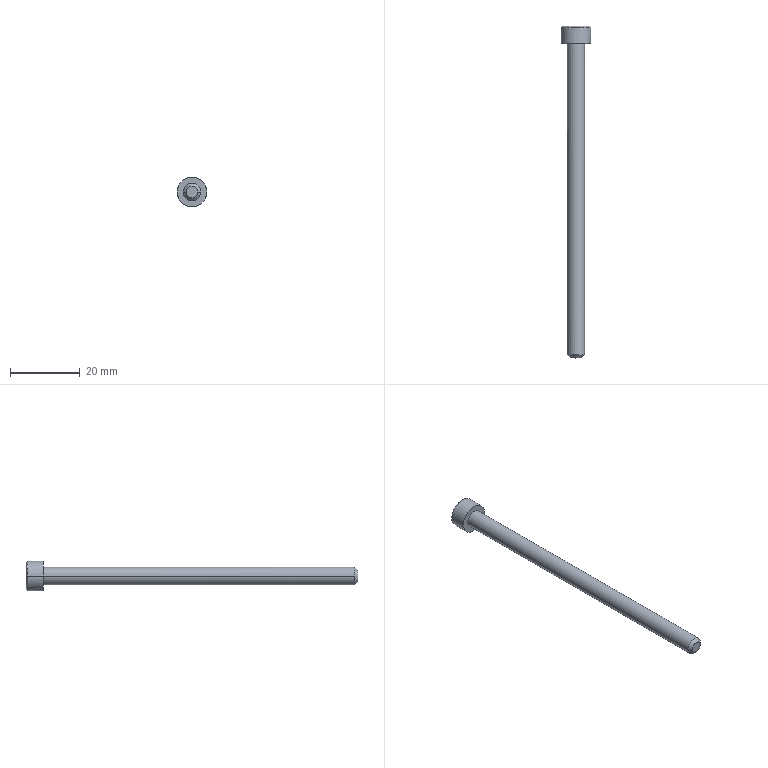Part | STEP file | BB62-M5-90L-6 | 1 solid | 18 faces | box 8.5 x 95 x 8.5 mm | volume 2008 mm3 | plane 10 | cylinder 4 | cone 4 | commonest cylinder face diameters 5 x2 8.5 x2
STEP:
#1=CARTESIAN_POINT('',(-4.25,0.,0.));
#2=VERTEX_POINT('',#1);
#3=CARTESIAN_POINT('',(4.25,0.,0.));
#4=VERTEX_POINT('',#3);
#5=CARTESIAN_POINT('',(0.,0.,0.));
#6=DIRECTION('',(0.,1.,0.));
#7=DIRECTION('',(-1.,0.,0.));
#8=AXIS2_PLACEMENT_3D('',#5,#6,#7);
#9=CIRCLE('',#8,4.25);
#10=EDGE_CURVE('',#2,#4,#9,.T.);
#11=ORIENTED_EDGE('',*,*,#10,.F.);
#12=CARTESIAN_POINT('',(0.,0.,0.));
#13=DIRECTION('',(0.,1.,0.));
#14=DIRECTION('',(1.,0.,0.));
#15=AXIS2_PLACEMENT_3D('',#12,#13,#14);
#16=CIRCLE('',#15,4.25);
#17=EDGE_CURVE('',#4,#2,#16,.T.);
#18=ORIENTED_EDGE('',*,*,#17,.F.);
#19=EDGE_LOOP('',(#11,#18));
#20=FACE_OUTER_BOUND('',#19,.T.);
#21=CARTESIAN_POINT('',(-2.5,0.,0.));
#22=VERTEX_POINT('',#21);
#23=CARTESIAN_POINT('',(2.5,0.,0.));
#24=VERTEX_POINT('',#23);
#25=CARTESIAN_POINT('',(0.,0.,0.));
#26=DIRECTION('',(0.,1.,0.));
#27=DIRECTION('',(-1.,0.,0.));
#28=AXIS2_PLACEMENT_3D('',#25,#26,#27);
#29=CIRCLE('',#28,2.5);
#30=EDGE_CURVE('',#22,#24,#29,.T.);
#31=ORIENTED_EDGE('',*,*,#30,.T.);
#32=CARTESIAN_POINT('',(0.,0.,0.));
#33=DIRECTION('',(0.,1.,0.));
#34=DIRECTION('',(1.,0.,0.));
#35=AXIS2_PLACEMENT_3D('',#32,#33,#34);
#36=CIRCLE('',#35,2.5);
#37=EDGE_CURVE('',#24,#22,#36,.T.);
#38=ORIENTED_EDGE('',*,*,#37,.T.);
#39=EDGE_LOOP('',(#31,#38));
#40=FACE_BOUND('',#39,.T.);
#41=CARTESIAN_POINT('',(-9.016,0.,9.016));
#42=DIRECTION('',(0.,1.,0.));
#43=DIRECTION('',(1.,0.,0.));
#44=AXIS2_PLACEMENT_3D('',#41,#42,#43);
#45=PLANE('',#44);
#46=ADVANCED_FACE('',(#20,#40),#45,.F.);
#47=CARTESIAN_POINT('',(4.25,4.7,0.));
#48=VERTEX_POINT('',#47);
#49=CARTESIAN_POINT('',(4.25,0.,0.));
#50=DIRECTION('',(0.,1.,0.));
#51=VECTOR('',#50,1000.);
#52=LINE('',#49,#51);
#53=EDGE_CURVE('',#4,#48,#52,.T.);
#54=ORIENTED_EDGE('',*,*,#53,.F.);
#55=ORIENTED_EDGE('',*,*,#17,.T.);
#56=CARTESIAN_POINT('',(-4.25,4.7,0.));
#57=VERTEX_POINT('',#56);
#58=CARTESIAN_POINT('',(-4.25,0.,0.));
#59=DIRECTION('',(0.,1.,0.));
#60=VECTOR('',#59,1000.);
#61=LINE('',#58,#60);
#62=EDGE_CURVE('',#2,#57,#61,.T.);
#63=ORIENTED_EDGE('',*,*,#62,.T.);
#64=CARTESIAN_POINT('',(4.25,4.7,0.));
#65=CARTESIAN_POINT('',(4.25,4.7,-0.5563));
#66=CARTESIAN_POINT('',(4.139,4.7,-1.112));
#67=CARTESIAN_POINT('',(3.714,4.7,-2.14));
#68=CARTESIAN_POINT('',(3.399,4.7,-2.612));
#69=CARTESIAN_POINT('',(2.612,4.7,-3.399));
#70=CARTESIAN_POINT('',(2.14,4.7,-3.714));
#71=CARTESIAN_POINT('',(1.112,4.7,-4.139));
#72=CARTESIAN_POINT('',(0.5563,4.7,-4.25));
#73=CARTESIAN_POINT('',(-0.5563,4.7,-4.25));
#74=CARTESIAN_POINT('',(-1.112,4.7,-4.139));
#75=CARTESIAN_POINT('',(-2.14,4.7,-3.714));
#76=CARTESIAN_POINT('',(-2.612,4.7,-3.399));
#77=CARTESIAN_POINT('',(-3.399,4.7,-2.612));
#78=CARTESIAN_POINT('',(-3.714,4.7,-2.14));
#79=CARTESIAN_POINT('',(-4.139,4.7,-1.112));
#80=CARTESIAN_POINT('',(-4.25,4.7,-0.5563));
#81=CARTESIAN_POINT('',(-4.25,4.7,0.));
#82=B_SPLINE_CURVE_WITH_KNOTS('',3,(#64,#65,#66,#67,#68,#69,#70,#71,#72,#73,#74,#75,#76,#77,#78,#79,#80,#81),.UNSPECIFIED.,.F.,.F.,(4,2,2,2,2,2,2,2,4),(0.,0.125,0.25,0.375,0.5,0.625,0.75,0.875,1.),.UNSPECIFIED.);
#83=EDGE_CURVE('',#48,#57,#82,.T.);
#84=ORIENTED_EDGE('',*,*,#83,.F.);
#85=EDGE_LOOP('',(#54,#55,#63,#84));
#86=FACE_OUTER_BOUND('',#85,.T.);
#87=CARTESIAN_POINT('',(0.,2.35,0.));
#88=DIRECTION('',(0.,1.,0.));
#89=DIRECTION('',(1.,0.,0.));
#90=AXIS2_PLACEMENT_3D('',#87,#88,#89);
#91=CYLINDRICAL_SURFACE('',#90,4.25);
#92=ADVANCED_FACE('',(#86),#91,.T.);
#93=CARTESIAN_POINT('',(3.73,5.,0.));
#94=VERTEX_POINT('',#93);
#95=CARTESIAN_POINT('',(3.73,5.,0.));
#96=CARTESIAN_POINT('',(3.904,4.9,0.));
#97=CARTESIAN_POINT('',(4.077,4.8,0.));
#98=CARTESIAN_POINT('',(4.25,4.7,0.));
#99=B_SPLINE_CURVE_WITH_KNOTS('',3,(#95,#96,#97,#98),.UNSPECIFIED.,.F.,.F.,(4,4),(0.,1.),.UNSPECIFIED.);
#100=EDGE_CURVE('',#94,#48,#99,.T.);
#101=ORIENTED_EDGE('',*,*,#100,.T.);
#102=ORIENTED_EDGE('',*,*,#83,.T.);
#103=CARTESIAN_POINT('',(-3.73,5.,0.));
#104=VERTEX_POINT('',#103);
#105=CARTESIAN_POINT('',(-3.73,5.,0.));
#106=CARTESIAN_POINT('',(-3.904,4.9,0.));
#107=CARTESIAN_POINT('',(-4.077,4.8,0.));
#108=CARTESIAN_POINT('',(-4.25,4.7,0.));
#109=B_SPLINE_CURVE_WITH_KNOTS('',3,(#105,#106,#107,#108),.UNSPECIFIED.,.F.,.F.,(4,4),(0.,1.),.UNSPECIFIED.);
#110=EDGE_CURVE('',#104,#57,#109,.T.);
#111=ORIENTED_EDGE('',*,*,#110,.F.);
#112=CARTESIAN_POINT('',(3.73,5.,0.));
#113=CARTESIAN_POINT('',(3.742,5.,-0.9708));
#114=CARTESIAN_POINT('',(3.325,5.,-1.947));
#115=CARTESIAN_POINT('',(2.293,5.,-2.984));
#116=CARTESIAN_POINT('',(1.881,5.,-3.259));
#117=CARTESIAN_POINT('',(0.9786,5.,-3.631));
#118=CARTESIAN_POINT('',(0.,5.,-3.829));
#119=CARTESIAN_POINT('',(-0.9786,5.,-3.631));
#120=CARTESIAN_POINT('',(-1.881,5.,-3.259));
#121=CARTESIAN_POINT('',(-2.293,5.,-2.984));
#122=CARTESIAN_POINT('',(-3.325,5.,-1.947));
#123=CARTESIAN_POINT('',(-3.742,5.,-0.9708));
#124=CARTESIAN_POINT('',(-3.73,5.,0.));
#125=B_SPLINE_CURVE_WITH_KNOTS('',3,(#112,#113,#114,#115,#116,#117,#118,#119,#120,#121,#122,#123,#124),.UNSPECIFIED.,.F.,.F.,(4,2,2,1,2,2,4),(0.,0.25,0.375,0.5,0.625,0.75,1.),.UNSPECIFIED.);
#126=EDGE_CURVE('',#94,#104,#125,.T.);
#127=ORIENTED_EDGE('',*,*,#126,.F.);
#128=EDGE_LOOP('',(#101,#102,#111,#127));
#129=FACE_OUTER_BOUND('',#128,.T.);
#130=CARTESIAN_POINT('',(0.,-992.846,0.));
#131=DIRECTION('',(0.,-1.,0.));
#132=DIRECTION('',(0.,0.,1.));
#133=AXIS2_PLACEMENT_3D('',#130,#131,#132);
#134=CONICAL_SURFACE('',#133,1731.952,1.047);
#135=ADVANCED_FACE('',(#129),#134,.T.);
#136=CARTESIAN_POINT('',(-3.73,5.,0.));
#137=CARTESIAN_POINT('',(-3.742,5.,0.9708));
#138=CARTESIAN_POINT('',(-3.325,5.,1.947));
#139=CARTESIAN_POINT('',(-2.293,5.,2.984));
#140=CARTESIAN_POINT('',(-1.881,5.,3.259));
#141=CARTESIAN_POINT('',(-0.9786,5.,3.631));
#142=CARTESIAN_POINT('',(0.,5.,3.829));
#143=CARTESIAN_POINT('',(0.9786,5.,3.631));
#144=CARTESIAN_POINT('',(1.881,5.,3.259));
#145=CARTESIAN_POINT('',(2.293,5.,2.984));
#146=CARTESIAN_POINT('',(3.325,5.,1.947));
#147=CARTESIAN_POINT('',(3.742,5.,0.9708));
#148=CARTESIAN_POINT('',(3.73,5.,0.));
#149=B_SPLINE_CURVE_WITH_KNOTS('',3,(#136,#137,#138,#139,#140,#141,#142,#143,#144,#145,#146,#147,#148),.UNSPECIFIED.,.F.,.F.,(4,2,2,1,2,2,4),(0.,0.25,0.375,0.5,0.625,0.75,1.),.UNSPECIFIED.);
#150=EDGE_CURVE('',#104,#94,#149,.T.);
#151=ORIENTED_EDGE('',*,*,#150,.T.);
#152=ORIENTED_EDGE('',*,*,#126,.T.);
#153=EDGE_LOOP('',(#151,#152));
#154=FACE_OUTER_BOUND('',#153,.T.);
#155=CARTESIAN_POINT('',(2.,5.,1.155));
#156=VERTEX_POINT('',#155);
#157=CARTESIAN_POINT('',(2.,5.,-1.155));
#158=VERTEX_POINT('',#157);
#159=CARTESIAN_POINT('',(2.,5.,1.155));
#160=DIRECTION('',(0.,0.,-1.));
#161=VECTOR('',#160,1000.);
#162=LINE('',#159,#161);
#163=EDGE_CURVE('',#156,#158,#162,.T.);
#164=ORIENTED_EDGE('',*,*,#163,.F.);
#165=CARTESIAN_POINT('',(0.,5.,2.309));
#166=VERTEX_POINT('',#165);
#167=CARTESIAN_POINT('',(0.,5.,2.309));
#168=DIRECTION('',(0.866,0.,-0.5));
#169=VECTOR('',#168,1000.);
#170=LINE('',#167,#169);
#171=EDGE_CURVE('',#166,#156,#170,.T.);
#172=ORIENTED_EDGE('',*,*,#171,.F.);
#173=CARTESIAN_POINT('',(-2.,5.,1.155));
#174=VERTEX_POINT('',#173);
#175=CARTESIAN_POINT('',(-2.,5.,1.155));
#176=DIRECTION('',(0.866,0.,0.5));
#177=VECTOR('',#176,1000.);
#178=LINE('',#175,#177);
#179=EDGE_CURVE('',#174,#166,#178,.T.);
#180=ORIENTED_EDGE('',*,*,#179,.F.);
#181=CARTESIAN_POINT('',(-2.,5.,-1.155));
#182=VERTEX_POINT('',#181);
#183=CARTESIAN_POINT('',(-2.,5.,-1.155));
#184=DIRECTION('',(0.,0.,1.));
#185=VECTOR('',#184,1000.);
#186=LINE('',#183,#185);
#187=EDGE_CURVE('',#182,#174,#186,.T.);
#188=ORIENTED_EDGE('',*,*,#187,.F.);
#189=CARTESIAN_POINT('',(0.,5.,-2.309));
#190=VERTEX_POINT('',#189);
#191=CARTESIAN_POINT('',(0.,5.,-2.309));
#192=DIRECTION('',(-0.866,0.,0.5));
#193=VECTOR('',#192,1000.);
#194=LINE('',#191,#193);
#195=EDGE_CURVE('',#190,#182,#194,.T.);
#196=ORIENTED_EDGE('',*,*,#195,.F.);
#197=CARTESIAN_POINT('',(2.,5.,-1.155));
#198=DIRECTION('',(-0.866,0.,-0.5));
#199=VECTOR('',#198,1000.);
#200=LINE('',#197,#199);
#201=EDGE_CURVE('',#158,#190,#200,.T.);
#202=ORIENTED_EDGE('',*,*,#201,.F.);
#203=EDGE_LOOP('',(#164,#172,#180,#188,#196,#202));
#204=FACE_BOUND('',#203,.T.);
#205=CARTESIAN_POINT('',(-7.913,5.,7.913));
#206=DIRECTION('',(0.,1.,0.));
#207=DIRECTION('',(1.,0.,0.));
#208=AXIS2_PLACEMENT_3D('',#205,#206,#207);
#209=PLANE('',#208);
#210=ADVANCED_FACE('',(#154,#204),#209,.T.);
#211=ORIENTED_EDGE('',*,*,#110,.T.);
#212=CARTESIAN_POINT('',(-4.25,4.7,0.));
#213=CARTESIAN_POINT('',(-4.25,4.7,0.5563));
#214=CARTESIAN_POINT('',(-4.139,4.7,1.112));
#215=CARTESIAN_POINT('',(-3.714,4.7,2.14));
#216=CARTESIAN_POINT('',(-3.399,4.7,2.612));
#217=CARTESIAN_POINT('',(-2.612,4.7,3.399));
#218=CARTESIAN_POINT('',(-2.14,4.7,3.714));
#219=CARTESIAN_POINT('',(-1.112,4.7,4.139));
#220=CARTESIAN_POINT('',(-0.5563,4.7,4.25));
#221=CARTESIAN_POINT('',(0.5563,4.7,4.25));
#222=CARTESIAN_POINT('',(1.112,4.7,4.139));
#223=CARTESIAN_POINT('',(2.14,4.7,3.714));
#224=CARTESIAN_POINT('',(2.612,4.7,3.399));
#225=CARTESIAN_POINT('',(3.399,4.7,2.612));
#226=CARTESIAN_POINT('',(3.714,4.7,2.14));
#227=CARTESIAN_POINT('',(4.139,4.7,1.112));
#228=CARTESIAN_POINT('',(4.25,4.7,0.5563));
#229=CARTESIAN_POINT('',(4.25,4.7,0.));
#230=B_SPLINE_CURVE_WITH_KNOTS('',3,(#212,#213,#214,#215,#216,#217,#218,#219,#220,#221,#222,#223,#224,#225,#226,#227,#228,#229),.UNSPECIFIED.,.F.,.F.,(4,2,2,2,2,2,2,2,4),(0.,0.125,0.25,0.375,0.5,0.625,0.75,0.875,1.),.UNSPECIFIED.);
#231=EDGE_CURVE('',#57,#48,#230,.T.);
#232=ORIENTED_EDGE('',*,*,#231,.T.);
#233=ORIENTED_EDGE('',*,*,#100,.F.);
#234=ORIENTED_EDGE('',*,*,#150,.F.);
#235=EDGE_LOOP('',(#211,#232,#233,#234));
#236=FACE_OUTER_BOUND('',#235,.T.);
#237=CARTESIAN_POINT('',(0.,-992.846,0.));
#238=DIRECTION('',(0.,-1.,0.));
#239=DIRECTION('',(0.,0.,-1.));
#240=AXIS2_PLACEMENT_3D('',#237,#238,#239);
#241=CONICAL_SURFACE('',#240,1731.952,1.047);
#242=ADVANCED_FACE('',(#236),#241,.T.);
#243=ORIENTED_EDGE('',*,*,#62,.F.);
#244=ORIENTED_EDGE('',*,*,#10,.T.);
#245=ORIENTED_EDGE('',*,*,#53,.T.);
#246=ORIENTED_EDGE('',*,*,#231,.F.);
#247=EDGE_LOOP('',(#243,#244,#245,#246));
#248=FACE_OUTER_BOUND('',#247,.T.);
#249=CARTESIAN_POINT('',(0.,2.35,0.));
#250=DIRECTION('',(0.,1.,0.));
#251=DIRECTION('',(1.,0.,0.));
#252=AXIS2_PLACEMENT_3D('',#249,#250,#251);
#253=CYLINDRICAL_SURFACE('',#252,4.25);
#254=ADVANCED_FACE('',(#248),#253,.T.);
#255=CARTESIAN_POINT('',(0.,2.5,-2.309));
#256=VERTEX_POINT('',#255);
#257=CARTESIAN_POINT('',(0.,5.,-2.309));
#258=DIRECTION('',(0.,-1.,0.));
#259=VECTOR('',#258,1000.);
#260=LINE('',#257,#259);
#261=EDGE_CURVE('',#190,#256,#260,.T.);
#262=ORIENTED_EDGE('',*,*,#261,.T.);
#263=CARTESIAN_POINT('',(2.,2.5,-1.155));
#264=VERTEX_POINT('',#263);
#265=CARTESIAN_POINT('',(2.,2.5,-1.155));
#266=DIRECTION('',(-0.866,0.,-0.5));
#267=VECTOR('',#266,1000.);
#268=LINE('',#265,#267);
#269=EDGE_CURVE('',#264,#256,#268,.T.);
#270=ORIENTED_EDGE('',*,*,#269,.F.);
#271=CARTESIAN_POINT('',(2.,5.,-1.155));
#272=DIRECTION('',(0.,-1.,0.));
#273=VECTOR('',#272,1000.);
#274=LINE('',#271,#273);
#275=EDGE_CURVE('',#158,#264,#274,.T.);
#276=ORIENTED_EDGE('',*,*,#275,.F.);
#277=ORIENTED_EDGE('',*,*,#201,.T.);
#278=EDGE_LOOP('',(#262,#270,#276,#277));
#279=FACE_OUTER_BOUND('',#278,.T.);
#280=CARTESIAN_POINT('',(3.211,1.197,-0.4558));
#281=DIRECTION('',(0.5,0.,-0.866));
#282=DIRECTION('',(-0.866,0.,-0.5));
#283=AXIS2_PLACEMENT_3D('',#280,#281,#282);
#284=PLANE('',#283);
#285=ADVANCED_FACE('',(#279),#284,.F.);
#286=ORIENTED_EDGE('',*,*,#275,.T.);
#287=CARTESIAN_POINT('',(2.,2.5,1.155));
#288=VERTEX_POINT('',#287);
#289=CARTESIAN_POINT('',(2.,2.5,1.155));
#290=DIRECTION('',(0.,0.,-1.));
#291=VECTOR('',#290,1000.);
#292=LINE('',#289,#291);
#293=EDGE_CURVE('',#288,#264,#292,.T.);
#294=ORIENTED_EDGE('',*,*,#293,.F.);
#295=CARTESIAN_POINT('',(2.,5.,1.155));
#296=DIRECTION('',(0.,-1.,0.));
#297=VECTOR('',#296,1000.);
#298=LINE('',#295,#297);
#299=EDGE_CURVE('',#156,#288,#298,.T.);
#300=ORIENTED_EDGE('',*,*,#299,.F.);
#301=ORIENTED_EDGE('',*,*,#163,.T.);
#302=EDGE_LOOP('',(#286,#294,#300,#301));
#303=FACE_OUTER_BOUND('',#302,.T.);
#304=CARTESIAN_POINT('',(2.,1.197,2.553));
#305=DIRECTION('',(1.,0.,0.));
#306=DIRECTION('',(0.,0.,-1.));
#307=AXIS2_PLACEMENT_3D('',#304,#305,#306);
#308=PLANE('',#307);
#309=ADVANCED_FACE('',(#303),#308,.F.);
#310=ORIENTED_EDGE('',*,*,#299,.T.);
#311=CARTESIAN_POINT('',(0.,2.5,2.309));
#312=VERTEX_POINT('',#311);
#313=CARTESIAN_POINT('',(0.,2.5,2.309));
#314=DIRECTION('',(0.866,0.,-0.5));
#315=VECTOR('',#314,1000.);
#316=LINE('',#313,#315);
#317=EDGE_CURVE('',#312,#288,#316,.T.);
#318=ORIENTED_EDGE('',*,*,#317,.F.);
#319=CARTESIAN_POINT('',(0.,5.,2.309));
#320=DIRECTION('',(0.,-1.,0.));
#321=VECTOR('',#320,1000.);
#322=LINE('',#319,#321);
#323=EDGE_CURVE('',#166,#312,#322,.T.);
#324=ORIENTED_EDGE('',*,*,#323,.F.);
#325=ORIENTED_EDGE('',*,*,#171,.T.);
#326=EDGE_LOOP('',(#310,#318,#324,#325));
#327=FACE_OUTER_BOUND('',#326,.T.);
#328=CARTESIAN_POINT('',(-1.211,1.197,3.008));
#329=DIRECTION('',(0.5,0.,0.866));
#330=DIRECTION('',(0.866,0.,-0.5));
#331=AXIS2_PLACEMENT_3D('',#328,#329,#330);
#332=PLANE('',#331);
#333=ADVANCED_FACE('',(#327),#332,.F.);
#334=ORIENTED_EDGE('',*,*,#323,.T.);
#335=CARTESIAN_POINT('',(-2.,2.5,1.155));
#336=VERTEX_POINT('',#335);
#337=CARTESIAN_POINT('',(-2.,2.5,1.155));
#338=DIRECTION('',(0.866,0.,0.5));
#339=VECTOR('',#338,1000.);
#340=LINE('',#337,#339);
#341=EDGE_CURVE('',#336,#312,#340,.T.);
#342=ORIENTED_EDGE('',*,*,#341,.F.);
#343=CARTESIAN_POINT('',(-2.,5.,1.155));
#344=DIRECTION('',(0.,-1.,0.));
#345=VECTOR('',#344,1000.);
#346=LINE('',#343,#345);
#347=EDGE_CURVE('',#174,#336,#346,.T.);
#348=ORIENTED_EDGE('',*,*,#347,.F.);
#349=ORIENTED_EDGE('',*,*,#179,.T.);
#350=EDGE_LOOP('',(#334,#342,#348,#349));
#351=FACE_OUTER_BOUND('',#350,.T.);
#352=CARTESIAN_POINT('',(-3.211,1.197,0.4558));
#353=DIRECTION('',(-0.5,0.,0.866));
#354=DIRECTION('',(0.866,0.,0.5));
#355=AXIS2_PLACEMENT_3D('',#352,#353,#354);
#356=PLANE('',#355);
#357=ADVANCED_FACE('',(#351),#356,.F.);
#358=ORIENTED_EDGE('',*,*,#347,.T.);
#359=CARTESIAN_POINT('',(-2.,2.5,-1.155));
#360=VERTEX_POINT('',#359);
#361=CARTESIAN_POINT('',(-2.,2.5,-1.155));
#362=DIRECTION('',(0.,0.,1.));
#363=VECTOR('',#362,1000.);
#364=LINE('',#361,#363);
#365=EDGE_CURVE('',#360,#336,#364,.T.);
#366=ORIENTED_EDGE('',*,*,#365,.F.);
#367=CARTESIAN_POINT('',(-2.,5.,-1.155));
#368=DIRECTION('',(0.,-1.,0.));
#369=VECTOR('',#368,1000.);
#370=LINE('',#367,#369);
#371=EDGE_CURVE('',#182,#360,#370,.T.);
#372=ORIENTED_EDGE('',*,*,#371,.F.);
#373=ORIENTED_EDGE('',*,*,#187,.T.);
#374=EDGE_LOOP('',(#358,#366,#372,#373));
#375=FACE_OUTER_BOUND('',#374,.T.);
#376=CARTESIAN_POINT('',(-2.,1.197,-2.553));
#377=DIRECTION('',(-1.,0.,0.));
#378=DIRECTION('',(0.,0.,1.));
#379=AXIS2_PLACEMENT_3D('',#376,#377,#378);
#380=PLANE('',#379);
#381=ADVANCED_FACE('',(#375),#380,.F.);
#382=ORIENTED_EDGE('',*,*,#371,.T.);
#383=CARTESIAN_POINT('',(0.,2.5,-2.309));
#384=DIRECTION('',(-0.866,0.,0.5));
#385=VECTOR('',#384,1000.);
#386=LINE('',#383,#385);
#387=EDGE_CURVE('',#256,#360,#386,.T.);
#388=ORIENTED_EDGE('',*,*,#387,.F.);
#389=ORIENTED_EDGE('',*,*,#261,.F.);
#390=ORIENTED_EDGE('',*,*,#195,.T.);
#391=EDGE_LOOP('',(#382,#388,#389,#390));
#392=FACE_OUTER_BOUND('',#391,.T.);
#393=CARTESIAN_POINT('',(1.211,1.197,-3.008));
#394=DIRECTION('',(-0.5,0.,-0.866));
#395=DIRECTION('',(-0.866,0.,0.5));
#396=AXIS2_PLACEMENT_3D('',#393,#394,#395);
#397=PLANE('',#396);
#398=ADVANCED_FACE('',(#392),#397,.F.);
#399=ORIENTED_EDGE('',*,*,#387,.T.);
#400=ORIENTED_EDGE('',*,*,#365,.T.);
#401=ORIENTED_EDGE('',*,*,#341,.T.);
#402=ORIENTED_EDGE('',*,*,#317,.T.);
#403=ORIENTED_EDGE('',*,*,#293,.T.);
#404=ORIENTED_EDGE('',*,*,#269,.T.);
#405=EDGE_LOOP('',(#399,#400,#401,#402,#403,#404));
#406=FACE_OUTER_BOUND('',#405,.T.);
#407=CARTESIAN_POINT('',(-4.583,2.5,4.583));
#408=DIRECTION('',(0.,1.,0.));
#409=DIRECTION('',(1.,0.,0.));
#410=AXIS2_PLACEMENT_3D('',#407,#408,#409);
#411=PLANE('',#410);
#412=ADVANCED_FACE('',(#406),#411,.T.);
#413=CARTESIAN_POINT('',(-2.5,-89.1,0.));
#414=VERTEX_POINT('',#413);
#415=CARTESIAN_POINT('',(-2.5,0.,0.));
#416=DIRECTION('',(0.,-1.,0.));
#417=VECTOR('',#416,1000.);
#418=LINE('',#415,#417);
#419=EDGE_CURVE('',#22,#414,#418,.T.);
#420=ORIENTED_EDGE('',*,*,#419,.F.);
#421=ORIENTED_EDGE('',*,*,#37,.F.);
#422=CARTESIAN_POINT('',(2.5,-89.1,0.));
#423=VERTEX_POINT('',#422);
#424=CARTESIAN_POINT('',(2.5,0.,0.));
#425=DIRECTION('',(0.,-1.,0.));
#426=VECTOR('',#425,1000.);
#427=LINE('',#424,#426);
#428=EDGE_CURVE('',#24,#423,#427,.T.);
#429=ORIENTED_EDGE('',*,*,#428,.T.);
#430=CARTESIAN_POINT('',(-2.5,-89.1,0.));
#431=CARTESIAN_POINT('',(-2.5,-89.1,-0.3272));
#432=CARTESIAN_POINT('',(-2.435,-89.1,-0.6544));
#433=CARTESIAN_POINT('',(-2.184,-89.1,-1.259));
#434=CARTESIAN_POINT('',(-1.999,-89.1,-1.536));
#435=CARTESIAN_POINT('',(-1.536,-89.1,-1.999));
#436=CARTESIAN_POINT('',(-1.259,-89.1,-2.184));
#437=CARTESIAN_POINT('',(-0.6544,-89.1,-2.435));
#438=CARTESIAN_POINT('',(-0.3272,-89.1,-2.5));
#439=CARTESIAN_POINT('',(0.3272,-89.1,-2.5));
#440=CARTESIAN_POINT('',(0.6544,-89.1,-2.435));
#441=CARTESIAN_POINT('',(1.259,-89.1,-2.184));
#442=CARTESIAN_POINT('',(1.536,-89.1,-1.999));
#443=CARTESIAN_POINT('',(1.999,-89.1,-1.536));
#444=CARTESIAN_POINT('',(2.184,-89.1,-1.259));
#445=CARTESIAN_POINT('',(2.435,-89.1,-0.6544));
#446=CARTESIAN_POINT('',(2.5,-89.1,-0.3272));
#447=CARTESIAN_POINT('',(2.5,-89.1,0.));
#448=B_SPLINE_CURVE_WITH_KNOTS('',3,(#430,#431,#432,#433,#434,#435,#436,#437,#438,#439,#440,#441,#442,#443,#444,#445,#446,#447),.UNSPECIFIED.,.F.,.F.,(4,2,2,2,2,2,2,2,4),(0.,0.125,0.25,0.375,0.5,0.625,0.75,0.875,1.),.UNSPECIFIED.);
#449=EDGE_CURVE('',#414,#423,#448,.T.);
#450=ORIENTED_EDGE('',*,*,#449,.F.);
#451=EDGE_LOOP('',(#420,#421,#429,#450));
#452=FACE_OUTER_BOUND('',#451,.T.);
#453=CARTESIAN_POINT('',(0.,-44.55,0.));
#454=DIRECTION('',(0.,1.,0.));
#455=DIRECTION('',(1.,0.,0.));
#456=AXIS2_PLACEMENT_3D('',#453,#454,#455);
#457=CYLINDRICAL_SURFACE('',#456,2.5);
#458=ADVANCED_FACE('',(#452),#457,.T.);
#459=CARTESIAN_POINT('',(-1.6,-90.,0.));
#460=VERTEX_POINT('',#459);
#461=CARTESIAN_POINT('',(-1.6,-90.,0.));
#462=CARTESIAN_POINT('',(-1.9,-89.7,0.));
#463=CARTESIAN_POINT('',(-2.2,-89.4,0.));
#464=CARTESIAN_POINT('',(-2.5,-89.1,0.));
#465=B_SPLINE_CURVE_WITH_KNOTS('',3,(#461,#462,#463,#464),.UNSPECIFIED.,.F.,.F.,(4,4),(0.,1.),.UNSPECIFIED.);
#466=EDGE_CURVE('',#460,#414,#465,.T.);
#467=ORIENTED_EDGE('',*,*,#466,.T.);
#468=ORIENTED_EDGE('',*,*,#449,.T.);
#469=CARTESIAN_POINT('',(1.6,-90.,0.));
#470=VERTEX_POINT('',#469);
#471=CARTESIAN_POINT('',(1.6,-90.,0.));
#472=CARTESIAN_POINT('',(1.9,-89.7,0.));
#473=CARTESIAN_POINT('',(2.2,-89.4,0.));
#474=CARTESIAN_POINT('',(2.5,-89.1,0.));
#475=B_SPLINE_CURVE_WITH_KNOTS('',3,(#471,#472,#473,#474),.UNSPECIFIED.,.F.,.F.,(4,4),(0.,1.),.UNSPECIFIED.);
#476=EDGE_CURVE('',#470,#423,#475,.T.);
#477=ORIENTED_EDGE('',*,*,#476,.F.);
#478=CARTESIAN_POINT('',(-1.6,-90.,0.));
#479=CARTESIAN_POINT('',(-1.602,-90.,-0.413));
#480=CARTESIAN_POINT('',(-1.434,-90.,-0.8264));
#481=CARTESIAN_POINT('',(-0.8448,-90.,-1.42));
#482=CARTESIAN_POINT('',(-0.4224,-90.,-1.6));
#483=CARTESIAN_POINT('',(0.4224,-90.,-1.6));
#484=CARTESIAN_POINT('',(0.8448,-90.,-1.42));
#485=CARTESIAN_POINT('',(1.434,-90.,-0.8264));
#486=CARTESIAN_POINT('',(1.602,-90.,-0.413));
#487=CARTESIAN_POINT('',(1.6,-90.,0.));
#488=B_SPLINE_CURVE_WITH_KNOTS('',3,(#478,#479,#480,#481,#482,#483,#484,#485,#486,#487),.UNSPECIFIED.,.F.,.F.,(4,2,2,2,4),(0.,0.25,0.5,0.75,1.),.UNSPECIFIED.);
#489=EDGE_CURVE('',#460,#470,#488,.T.);
#490=ORIENTED_EDGE('',*,*,#489,.F.);
#491=EDGE_LOOP('',(#467,#468,#477,#490));
#492=FACE_OUTER_BOUND('',#491,.T.);
#493=CARTESIAN_POINT('',(0.,908.4,0.));
#494=DIRECTION('',(0.,1.,0.));
#495=DIRECTION('',(0.,0.,1.));
#496=AXIS2_PLACEMENT_3D('',#493,#494,#495);
#497=CONICAL_SURFACE('',#496,999.967,0.7854);
#498=ADVANCED_FACE('',(#492),#497,.T.);
#499=ORIENTED_EDGE('',*,*,#489,.T.);
#500=CARTESIAN_POINT('',(1.6,-90.,0.));
#501=CARTESIAN_POINT('',(1.602,-90.,0.413));
#502=CARTESIAN_POINT('',(1.434,-90.,0.8264));
#503=CARTESIAN_POINT('',(0.8448,-90.,1.42));
#504=CARTESIAN_POINT('',(0.4224,-90.,1.6));
#505=CARTESIAN_POINT('',(-0.4224,-90.,1.6));
#506=CARTESIAN_POINT('',(-0.8448,-90.,1.42));
#507=CARTESIAN_POINT('',(-1.434,-90.,0.8264));
#508=CARTESIAN_POINT('',(-1.602,-90.,0.413));
#509=CARTESIAN_POINT('',(-1.6,-90.,0.));
#510=B_SPLINE_CURVE_WITH_KNOTS('',3,(#500,#501,#502,#503,#504,#505,#506,#507,#508,#509),.UNSPECIFIED.,.F.,.F.,(4,2,2,2,4),(0.,0.25,0.5,0.75,1.),.UNSPECIFIED.);
#511=EDGE_CURVE('',#470,#460,#510,.T.);
#512=ORIENTED_EDGE('',*,*,#511,.T.);
#513=EDGE_LOOP('',(#499,#512));
#514=FACE_OUTER_BOUND('',#513,.T.);
#515=CARTESIAN_POINT('',(-3.394,-90.,3.394));
#516=DIRECTION('',(0.,1.,0.));
#517=DIRECTION('',(1.,0.,0.));
#518=AXIS2_PLACEMENT_3D('',#515,#516,#517);
#519=PLANE('',#518);
#520=ADVANCED_FACE('',(#514),#519,.F.);
#521=ORIENTED_EDGE('',*,*,#476,.T.);
#522=CARTESIAN_POINT('',(2.5,-89.1,0.));
#523=CARTESIAN_POINT('',(2.5,-89.1,0.3272));
#524=CARTESIAN_POINT('',(2.435,-89.1,0.6544));
#525=CARTESIAN_POINT('',(2.184,-89.1,1.259));
#526=CARTESIAN_POINT('',(1.999,-89.1,1.536));
#527=CARTESIAN_POINT('',(1.536,-89.1,1.999));
#528=CARTESIAN_POINT('',(1.259,-89.1,2.184));
#529=CARTESIAN_POINT('',(0.6544,-89.1,2.435));
#530=CARTESIAN_POINT('',(0.3272,-89.1,2.5));
#531=CARTESIAN_POINT('',(-0.3272,-89.1,2.5));
#532=CARTESIAN_POINT('',(-0.6544,-89.1,2.435));
#533=CARTESIAN_POINT('',(-1.259,-89.1,2.184));
#534=CARTESIAN_POINT('',(-1.536,-89.1,1.999));
#535=CARTESIAN_POINT('',(-1.999,-89.1,1.536));
#536=CARTESIAN_POINT('',(-2.184,-89.1,1.259));
#537=CARTESIAN_POINT('',(-2.435,-89.1,0.6544));
#538=CARTESIAN_POINT('',(-2.5,-89.1,0.3272));
#539=CARTESIAN_POINT('',(-2.5,-89.1,0.));
#540=B_SPLINE_CURVE_WITH_KNOTS('',3,(#522,#523,#524,#525,#526,#527,#528,#529,#530,#531,#532,#533,#534,#535,#536,#537,#538,#539),.UNSPECIFIED.,.F.,.F.,(4,2,2,2,2,2,2,2,4),(0.,0.125,0.25,0.375,0.5,0.625,0.75,0.875,1.),.UNSPECIFIED.);
#541=EDGE_CURVE('',#423,#414,#540,.T.);
#542=ORIENTED_EDGE('',*,*,#541,.T.);
#543=ORIENTED_EDGE('',*,*,#466,.F.);
#544=ORIENTED_EDGE('',*,*,#511,.F.);
#545=EDGE_LOOP('',(#521,#542,#543,#544));
#546=FACE_OUTER_BOUND('',#545,.T.);
#547=CARTESIAN_POINT('',(0.,908.4,0.));
#548=DIRECTION('',(0.,1.,0.));
#549=DIRECTION('',(0.,0.,-1.));
#550=AXIS2_PLACEMENT_3D('',#547,#548,#549);
#551=CONICAL_SURFACE('',#550,999.967,0.7854);
#552=ADVANCED_FACE('',(#546),#551,.T.);
#553=ORIENTED_EDGE('',*,*,#428,.F.);
#554=ORIENTED_EDGE('',*,*,#30,.F.);
#555=ORIENTED_EDGE('',*,*,#419,.T.);
#556=ORIENTED_EDGE('',*,*,#541,.F.);
#557=EDGE_LOOP('',(#553,#554,#555,#556));
#558=FACE_OUTER_BOUND('',#557,.T.);
#559=CARTESIAN_POINT('',(0.,-44.55,0.));
#560=DIRECTION('',(0.,1.,0.));
#561=DIRECTION('',(1.,0.,0.));
#562=AXIS2_PLACEMENT_3D('',#559,#560,#561);
#563=CYLINDRICAL_SURFACE('',#562,2.5);
#564=ADVANCED_FACE('',(#558),#563,.T.);
#565=CLOSED_SHELL('',(#46,#92,#135,#210,#242,#254,#285,#309,#333,#357,#381,#398,#412,#458,#498,#520,#552,#564));
#566=MANIFOLD_SOLID_BREP('',#565);
#567=CARTESIAN_POINT('',(0.,0.,0.));
#568=DIRECTION('',(0.,0.,1.));
#569=DIRECTION('',(1.,0.,0.));
#570=AXIS2_PLACEMENT_3D('',#567,#568,#569);
#571=(LENGTH_UNIT()NAMED_UNIT(*)SI_UNIT(.MILLI.,.METRE.));
#572=UNCERTAINTY_MEASURE_WITH_UNIT(LENGTH_MEASURE(0.00001),#571,'','');
#573=(NAMED_UNIT(*)PLANE_ANGLE_UNIT()SI_UNIT($,.RADIAN.));
#574=(NAMED_UNIT(*)SI_UNIT($,.STERADIAN.)SOLID_ANGLE_UNIT());
#575=(GEOMETRIC_REPRESENTATION_CONTEXT(3)GLOBAL_UNCERTAINTY_ASSIGNED_CONTEXT((#572))GLOBAL_UNIT_ASSIGNED_CONTEXT((#571,#573,#574))REPRESENTATION_CONTEXT('',''));
#576=ADVANCED_BREP_SHAPE_REPRESENTATION('',(#566,#570),#575);